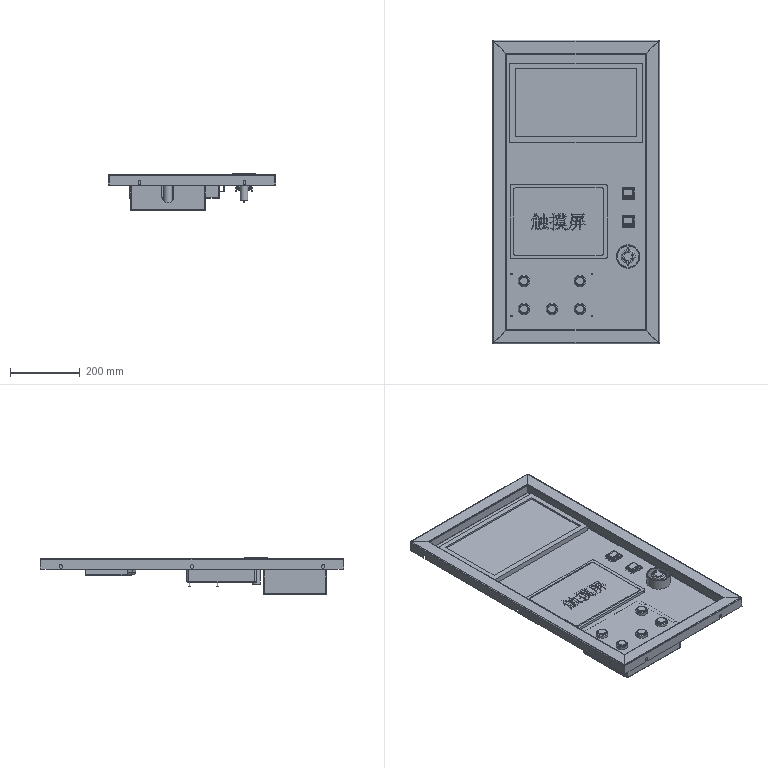Part | NX | 17 solids | 1235 faces | box 478 x 869 x 103.5 mm | volume 5270111 mm3 | plane 733 | cylinder 305 | spline 104 | cone 67 | torus 18 | sphere 8 | commonest cylinder face diameters 1 x32 1.473 x20 4 x20 2 x16 5.473 x14 5 x10